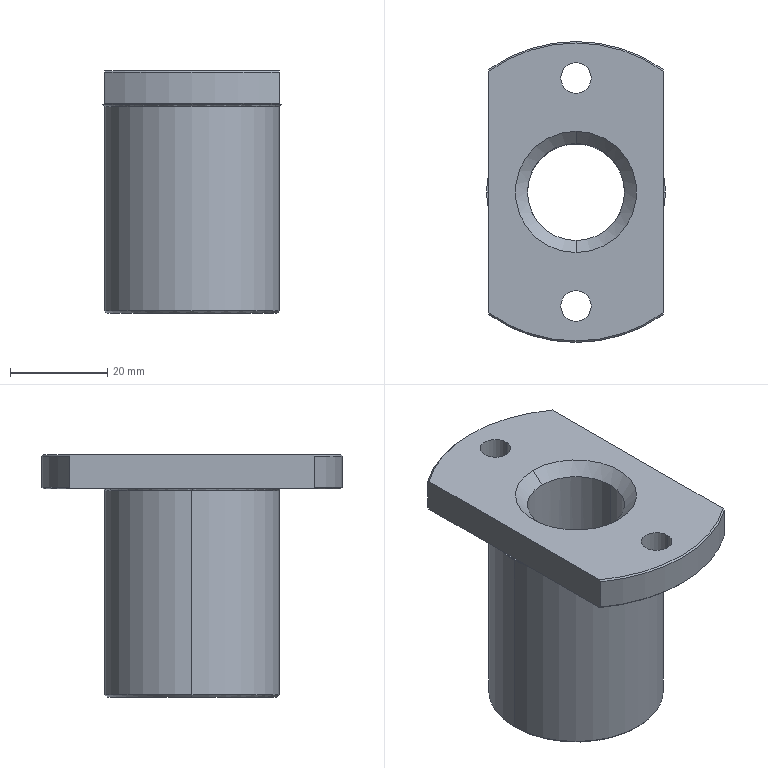Part | SolidWorks | features BaseBody 1 | 1 solid | 30 faces | box 36.8 x 62 x 50 mm | volume 41876 mm3 | cylinder 10 | cone 10 | plane 8 | spline 2 | commonest cylinder face diameters 6.3 x4 20 x2 36 x2 62 x2
STEP:
#1=CARTESIAN_POINT('',(18.4,0.,-7.));
#2=VERTEX_POINT('',#1);
#3=CARTESIAN_POINT('',(18.,3.816,-7.));
#4=VERTEX_POINT('',#3);
#5=CARTESIAN_POINT('',(18.4,0.,-7.));
#6=CARTESIAN_POINT('',(18.4,1.286,-7.));
#7=CARTESIAN_POINT('',(18.267,2.558,-7.));
#8=CARTESIAN_POINT('',(18.,3.816,-7.));
#9=B_SPLINE_CURVE_WITH_KNOTS('',3,(#5,#6,#7,#8),.UNSPECIFIED.,.F.,.F.,(4,4),(0.5,1.),.UNSPECIFIED.);
#10=EDGE_CURVE('',#2,#4,#9,.T.);
#11=ORIENTED_EDGE('',*,*,#10,.F.);
#12=CARTESIAN_POINT('',(18.,0.,-7.4));
#13=VERTEX_POINT('',#12);
#14=CARTESIAN_POINT('',(18.4,0.,-7.4));
#15=DIRECTION('',(0.,-1.,0.));
#16=DIRECTION('',(1.,0.,0.));
#17=AXIS2_PLACEMENT_3D('',#14,#15,#16);
#18=CIRCLE('',#17,0.4);
#19=EDGE_CURVE('',#2,#13,#18,.T.);
#20=ORIENTED_EDGE('',*,*,#19,.T.);
#21=CARTESIAN_POINT('',(-18.,0.,-7.4));
#22=VERTEX_POINT('',#21);
#23=CARTESIAN_POINT('',(0.,0.,-7.4));
#24=DIRECTION('',(0.,0.,-1.));
#25=DIRECTION('',(1.,0.,0.));
#26=AXIS2_PLACEMENT_3D('',#23,#24,#25);
#27=CIRCLE('',#26,18.);
#28=EDGE_CURVE('',#22,#13,#27,.T.);
#29=ORIENTED_EDGE('',*,*,#28,.F.);
#30=CARTESIAN_POINT('',(-18.4,0.,-7.));
#31=VERTEX_POINT('',#30);
#32=CARTESIAN_POINT('',(-18.4,0.,-7.4));
#33=DIRECTION('',(0.,1.,0.));
#34=DIRECTION('',(-1.,0.,0.));
#35=AXIS2_PLACEMENT_3D('',#32,#33,#34);
#36=CIRCLE('',#35,0.4);
#37=EDGE_CURVE('',#31,#22,#36,.T.);
#38=ORIENTED_EDGE('',*,*,#37,.F.);
#39=CARTESIAN_POINT('',(-18.,3.816,-7.));
#40=VERTEX_POINT('',#39);
#41=CARTESIAN_POINT('',(-18.,3.816,-7.));
#42=CARTESIAN_POINT('',(-18.267,2.558,-7.));
#43=CARTESIAN_POINT('',(-18.4,1.286,-7.));
#44=CARTESIAN_POINT('',(-18.4,0.,-7.));
#45=B_SPLINE_CURVE_WITH_KNOTS('',3,(#41,#42,#43,#44),.UNSPECIFIED.,.F.,.F.,(4,4),(0.,0.5),.UNSPECIFIED.);
#46=EDGE_CURVE('',#40,#31,#45,.T.);
#47=ORIENTED_EDGE('',*,*,#46,.F.);
#48=CARTESIAN_POINT('',(18.,3.816,-7.));
#49=CARTESIAN_POINT('',(17.897,4.302,-7.));
#50=CARTESIAN_POINT('',(17.714,5.022,-7.));
#51=CARTESIAN_POINT('',(17.45,5.846,-7.));
#52=CARTESIAN_POINT('',(17.305,6.255,-7.));
#53=CARTESIAN_POINT('',(17.229,6.458,-7.));
#54=CARTESIAN_POINT('',(17.196,6.545,-7.));
#55=CARTESIAN_POINT('',(17.174,6.603,-7.));
#56=CARTESIAN_POINT('',(17.164,6.631,-7.));
#57=CARTESIAN_POINT('',(16.964,7.145,-7.));
#58=CARTESIAN_POINT('',(16.653,7.856,-7.));
#59=CARTESIAN_POINT('',(16.238,8.66,-7.));
#60=CARTESIAN_POINT('',(16.018,9.056,-7.));
#61=CARTESIAN_POINT('',(15.921,9.224,-7.));
#62=CARTESIAN_POINT('',(15.856,9.336,-7.));
#63=CARTESIAN_POINT('',(15.824,9.39,-7.));
#64=CARTESIAN_POINT('',(15.515,9.907,-7.));
#65=CARTESIAN_POINT('',(15.074,10.575,-7.));
#66=CARTESIAN_POINT('',(14.511,11.318,-7.));
#67=CARTESIAN_POINT('',(14.26,11.629,-7.));
#68=CARTESIAN_POINT('',(14.089,11.835,-7.));
#69=CARTESIAN_POINT('',(14.005,11.935,-7.));
#70=CARTESIAN_POINT('',(13.205,12.86,-7.));
#71=CARTESIAN_POINT('',(12.428,13.612,-7.));
#72=CARTESIAN_POINT('',(11.161,14.638,-7.));
#73=CARTESIAN_POINT('',(10.508,15.122,-7.));
#74=CARTESIAN_POINT('',(9.711,15.633,-7.));
#75=CARTESIAN_POINT('',(9.362,15.841,-7.));
#76=CARTESIAN_POINT('',(9.127,15.977,-7.));
#77=CARTESIAN_POINT('',(9.008,16.045,-7.));
#78=CARTESIAN_POINT('',(8.422,16.368,-7.));
#79=CARTESIAN_POINT('',(7.705,16.724,-7.));
#80=CARTESIAN_POINT('',(6.845,17.083,-7.));
#81=CARTESIAN_POINT('',(6.408,17.249,-7.));
#82=CARTESIAN_POINT('',(6.22,17.317,-7.));
#83=CARTESIAN_POINT('',(6.094,17.362,-7.));
#84=CARTESIAN_POINT('',(6.029,17.384,-7.));
#85=CARTESIAN_POINT('',(5.477,17.574,-7.));
#86=CARTESIAN_POINT('',(4.733,17.794,-7.));
#87=CARTESIAN_POINT('',(3.851,17.996,-7.));
#88=CARTESIAN_POINT('',(3.406,18.083,-7.));
#89=CARTESIAN_POINT('',(3.183,18.123,-7.));
#90=CARTESIAN_POINT('',(3.087,18.139,-7.));
#91=CARTESIAN_POINT('',(3.023,18.15,-7.));
#92=CARTESIAN_POINT('',(2.99,18.155,-7.));
#93=CARTESIAN_POINT('',(1.979,18.32,-7.));
#94=CARTESIAN_POINT('',(0.9933,18.4,-7.));
#95=CARTESIAN_POINT('',(-0.4967,18.4,-7.));
#96=CARTESIAN_POINT('',(-1.239,18.37,-7.));
#97=CARTESIAN_POINT('',(-2.101,18.283,-7.));
#98=CARTESIAN_POINT('',(-2.531,18.226,-7.));
#99=CARTESIAN_POINT('',(-2.745,18.194,-7.));
#100=CARTESIAN_POINT('',(-2.837,18.18,-7.));
#101=CARTESIAN_POINT('',(-2.898,18.17,-7.));
#102=CARTESIAN_POINT('',(-2.927,18.166,-7.));
#103=CARTESIAN_POINT('',(-3.472,18.077,-7.));
#104=CARTESIAN_POINT('',(-4.232,17.92,-7.));
#105=CARTESIAN_POINT('',(-5.105,17.681,-7.));
#106=CARTESIAN_POINT('',(-5.537,17.548,-7.));
#107=CARTESIAN_POINT('',(-5.722,17.488,-7.));
#108=CARTESIAN_POINT('',(-5.845,17.447,-7.));
#109=CARTESIAN_POINT('',(-5.905,17.427,-7.));
#110=CARTESIAN_POINT('',(-6.474,17.232,-7.));
#111=CARTESIAN_POINT('',(-7.219,16.94,-7.));
#112=CARTESIAN_POINT('',(-8.063,16.543,-7.));
#113=CARTESIAN_POINT('',(-8.419,16.361,-7.));
#114=CARTESIAN_POINT('',(-8.656,16.237,-7.));
#115=CARTESIAN_POINT('',(-8.771,16.175,-7.));
#116=CARTESIAN_POINT('',(-9.842,15.585,-7.));
#117=CARTESIAN_POINT('',(-10.739,14.981,-7.));
#118=CARTESIAN_POINT('',(-12.006,13.954,-7.));
#119=CARTESIAN_POINT('',(-12.614,13.415,-7.));
#120=CARTESIAN_POINT('',(-13.279,12.742,-7.));
#121=CARTESIAN_POINT('',(-13.555,12.443,-7.));
#122=CARTESIAN_POINT('',(-13.737,12.242,-7.));
#123=CARTESIAN_POINT('',(-13.828,12.139,-7.));
#124=CARTESIAN_POINT('',(-14.266,11.633,-7.));
#125=CARTESIAN_POINT('',(-14.762,11.006,-7.));
#126=CARTESIAN_POINT('',(-15.292,10.239,-7.));
#127=CARTESIAN_POINT('',(-15.545,9.846,-7.));
#128=CARTESIAN_POINT('',(-15.651,9.676,-7.));
#129=CARTESIAN_POINT('',(-15.72,9.562,-7.));
#130=CARTESIAN_POINT('',(-15.756,9.503,-7.));
#131=CARTESIAN_POINT('',(-16.056,9.002,-7.));
#132=CARTESIAN_POINT('',(-16.426,8.32,-7.));
#133=CARTESIAN_POINT('',(-16.806,7.499,-7.));
#134=CARTESIAN_POINT('',(-16.983,7.082,-7.));
#135=CARTESIAN_POINT('',(-17.069,6.872,-7.));
#136=CARTESIAN_POINT('',(-17.105,6.782,-7.));
#137=CARTESIAN_POINT('',(-17.128,6.722,-7.));
#138=CARTESIAN_POINT('',(-17.141,6.69,-7.));
#139=CARTESIAN_POINT('',(-17.511,5.735,-7.));
#140=CARTESIAN_POINT('',(-17.794,4.787,-7.));
#141=CARTESIAN_POINT('',(-18.,3.816,-7.));
#142=B_SPLINE_CURVE_WITH_KNOTS('',3,(#48,#49,#50,#51,#52,#53,#54,#55,#56,#57,#58,#59,#60,#61,#62,#63,#64,#65,#66,#67,#68,#69,#70,#71,#72,#73,#74,#75,#76,#77,#78,#79,#80,#81,#82,#83,#84,#85,#86,#87,#88,#89,#90,#91,#92,#93,#94,#95,#96,#97,#98,#99,#100,#101,#102,#103,#104,#105,#106,#107,#108,#109,#110,#111,#112,#113,#114,#115,#116,#117,#118,#119,#120,#121,#122,#123,#124,#125,#126,#127,#128,#129,#130,#131,#132,#133,#134,#135,#136,#137,#138,#139,#140,#141),.UNSPECIFIED.,.F.,.F.,(4,1,1,1,1,2,2,1,1,1,2,2,1,1,2,2,2,1,1,2,2,1,1,1,2,2,1,1,1,1,2,2,2,1,1,1,1,2,2,1,1,1,2,2,1,1,2,2,2,1,1,2,2,1,1,1,2,2,1,1,1,1,2,2,4),(0.,0.03125,0.04687,0.05469,0.05859,0.06055,0.0625,0.09375,0.1094,0.1172,0.1211,0.125,0.1562,0.1719,0.1797,0.1875,0.25,0.2812,0.2969,0.3047,0.3125,0.3437,0.3594,0.3672,0.3711,0.375,0.4063,0.4219,0.4297,0.4336,0.4355,0.4375,0.5,0.5313,0.5469,0.5547,0.5586,0.5605,0.5625,0.5938,0.6094,0.6172,0.6211,0.625,0.6563,0.6719,0.6797,0.6875,0.75,0.7813,0.7969,0.8047,0.8125,0.8438,0.8594,0.8672,0.8711,0.875,0.9063,0.9219,0.9297,0.9336,0.9355,0.9375,1.),.UNSPECIFIED.);
#143=EDGE_CURVE('',#4,#40,#142,.T.);
#144=ORIENTED_EDGE('',*,*,#143,.F.);
#145=EDGE_LOOP('',(#11,#20,#29,#38,#47,#144));
#146=FACE_OUTER_BOUND('',#145,.T.);
#147=CARTESIAN_POINT('',(-18.4,0.,-7.));
#148=CARTESIAN_POINT('',(-18.4,36.8,-7.));
#149=CARTESIAN_POINT('',(18.4,36.8,-7.));
#150=CARTESIAN_POINT('',(18.4,0.,-7.));
#151=CARTESIAN_POINT('',(-18.166,0.,-7.));
#152=CARTESIAN_POINT('',(-18.166,36.331,-7.));
#153=CARTESIAN_POINT('',(18.166,36.331,-7.));
#154=CARTESIAN_POINT('',(18.166,0.,-7.));
#155=CARTESIAN_POINT('',(-18.,0.,-7.166));
#156=CARTESIAN_POINT('',(-18.,36.,-7.166));
#157=CARTESIAN_POINT('',(18.,36.,-7.166));
#158=CARTESIAN_POINT('',(18.,0.,-7.166));
#159=CARTESIAN_POINT('',(-18.,0.,-7.4));
#160=CARTESIAN_POINT('',(-18.,36.,-7.4));
#161=CARTESIAN_POINT('',(18.,36.,-7.4));
#162=CARTESIAN_POINT('',(18.,0.,-7.4));
#163=(BOUNDED_SURFACE()B_SPLINE_SURFACE(3,3,((#147,#148,#149,#150),(#151,#152,#153,#154),(#155,#156,#157,#158),(#159,#160,#161,#162)),.UNSPECIFIED.,.F.,.F.,.F.)B_SPLINE_SURFACE_WITH_KNOTS((4,4),(4,4),(0.,1.),(0.,1.),.UNSPECIFIED.)GEOMETRIC_REPRESENTATION_ITEM()RATIONAL_B_SPLINE_SURFACE(((1.,0.3333,0.3333,1.),(0.8047,0.2682,0.2682,0.8047),(0.8047,0.2682,0.2682,0.8047),(1.,0.3333,0.3333,1.)))REPRESENTATION_ITEM('')SURFACE());
#164=ADVANCED_FACE('',(#146),#163,.F.);
#165=CARTESIAN_POINT('',(18.,0.,-49.5));
#166=VERTEX_POINT('',#165);
#167=CARTESIAN_POINT('',(-18.,0.,-49.5));
#168=VERTEX_POINT('',#167);
#169=CARTESIAN_POINT('',(0.,0.,-49.5));
#170=DIRECTION('',(0.,0.,1.));
#171=DIRECTION('',(1.,0.,0.));
#172=AXIS2_PLACEMENT_3D('',#169,#170,#171);
#173=CIRCLE('',#172,18.);
#174=EDGE_CURVE('',#166,#168,#173,.T.);
#175=ORIENTED_EDGE('',*,*,#174,.T.);
#176=CARTESIAN_POINT('',(-18.,0.,-50.));
#177=DIRECTION('',(0.,0.,1.));
#178=VECTOR('',#177,1000.);
#179=LINE('',#176,#178);
#180=EDGE_CURVE('',#168,#22,#179,.T.);
#181=ORIENTED_EDGE('',*,*,#180,.T.);
#182=ORIENTED_EDGE('',*,*,#28,.T.);
#183=CARTESIAN_POINT('',(18.,0.,-50.));
#184=DIRECTION('',(0.,0.,1.));
#185=VECTOR('',#184,1000.);
#186=LINE('',#183,#185);
#187=EDGE_CURVE('',#166,#13,#186,.T.);
#188=ORIENTED_EDGE('',*,*,#187,.F.);
#189=EDGE_LOOP('',(#175,#181,#182,#188));
#190=FACE_OUTER_BOUND('',#189,.T.);
#191=CARTESIAN_POINT('',(0.,0.,-50.));
#192=DIRECTION('',(0.,0.,1.));
#193=DIRECTION('',(1.,0.,0.));
#194=AXIS2_PLACEMENT_3D('',#191,#192,#193);
#195=CYLINDRICAL_SURFACE('',#194,18.);
#196=ADVANCED_FACE('',(#190),#195,.T.);
#197=CARTESIAN_POINT('',(17.5,0.,-50.));
#198=VERTEX_POINT('',#197);
#199=CARTESIAN_POINT('',(-17.5,0.,-50.));
#200=VERTEX_POINT('',#199);
#201=CARTESIAN_POINT('',(0.,0.,-50.));
#202=DIRECTION('',(0.,0.,1.));
#203=DIRECTION('',(1.,0.,0.));
#204=AXIS2_PLACEMENT_3D('',#201,#202,#203);
#205=CIRCLE('',#204,17.5);
#206=EDGE_CURVE('',#198,#200,#205,.T.);
#207=ORIENTED_EDGE('',*,*,#206,.T.);
#208=CARTESIAN_POINT('',(-18.,0.,-49.5));
#209=DIRECTION('',(-0.7071,0.,0.7071));
#210=VECTOR('',#209,1000.);
#211=LINE('',#208,#210);
#212=EDGE_CURVE('',#200,#168,#211,.T.);
#213=ORIENTED_EDGE('',*,*,#212,.T.);
#214=ORIENTED_EDGE('',*,*,#174,.F.);
#215=CARTESIAN_POINT('',(18.,0.,-49.5));
#216=DIRECTION('',(0.7071,0.,0.7071));
#217=VECTOR('',#216,1000.);
#218=LINE('',#215,#217);
#219=EDGE_CURVE('',#198,#166,#218,.T.);
#220=ORIENTED_EDGE('',*,*,#219,.F.);
#221=EDGE_LOOP('',(#207,#213,#214,#220));
#222=FACE_OUTER_BOUND('',#221,.T.);
#223=CARTESIAN_POINT('',(0.,0.,-49.5));
#224=DIRECTION('',(0.,0.,1.));
#225=DIRECTION('',(1.,0.,0.));
#226=AXIS2_PLACEMENT_3D('',#223,#224,#225);
#227=CONICAL_SURFACE('',#226,18.,0.7854);
#228=ADVANCED_FACE('',(#222),#227,.T.);
#229=CARTESIAN_POINT('',(3.15,23.5,0.));
#230=VERTEX_POINT('',#229);
#231=CARTESIAN_POINT('',(-3.15,23.5,0.));
#232=VERTEX_POINT('',#231);
#233=CARTESIAN_POINT('',(0.,23.5,0.));
#234=DIRECTION('',(0.,0.,-1.));
#235=DIRECTION('',(-1.,0.,0.));
#236=AXIS2_PLACEMENT_3D('',#233,#234,#235);
#237=CIRCLE('',#236,3.15);
#238=EDGE_CURVE('',#230,#232,#237,.T.);
#239=ORIENTED_EDGE('',*,*,#238,.F.);
#240=CARTESIAN_POINT('',(3.15,23.5,-7.));
#241=VERTEX_POINT('',#240);
#242=CARTESIAN_POINT('',(3.15,23.5,-7.));
#243=DIRECTION('',(0.,0.,-1.));
#244=VECTOR('',#243,1000.);
#245=LINE('',#242,#244);
#246=EDGE_CURVE('',#230,#241,#245,.T.);
#247=ORIENTED_EDGE('',*,*,#246,.T.);
#248=CARTESIAN_POINT('',(-3.15,23.5,-7.));
#249=VERTEX_POINT('',#248);
#250=CARTESIAN_POINT('',(0.,23.5,-7.));
#251=DIRECTION('',(0.,0.,-1.));
#252=DIRECTION('',(-1.,0.,0.));
#253=AXIS2_PLACEMENT_3D('',#250,#251,#252);
#254=CIRCLE('',#253,3.15);
#255=EDGE_CURVE('',#241,#249,#254,.T.);
#256=ORIENTED_EDGE('',*,*,#255,.T.);
#257=CARTESIAN_POINT('',(-3.15,23.5,-7.));
#258=DIRECTION('',(0.,0.,-1.));
#259=VECTOR('',#258,1000.);
#260=LINE('',#257,#259);
#261=EDGE_CURVE('',#232,#249,#260,.T.);
#262=ORIENTED_EDGE('',*,*,#261,.F.);
#263=EDGE_LOOP('',(#239,#247,#256,#262));
#264=FACE_OUTER_BOUND('',#263,.T.);
#265=CARTESIAN_POINT('',(0.,23.5,-7.));
#266=DIRECTION('',(0.,0.,-1.));
#267=DIRECTION('',(-1.,0.,0.));
#268=AXIS2_PLACEMENT_3D('',#265,#266,#267);
#269=CYLINDRICAL_SURFACE('',#268,3.15);
#270=ADVANCED_FACE('',(#264),#269,.F.);
#271=CARTESIAN_POINT('',(3.15,-23.5,0.));
#272=VERTEX_POINT('',#271);
#273=CARTESIAN_POINT('',(-3.15,-23.5,0.));
#274=VERTEX_POINT('',#273);
#275=CARTESIAN_POINT('',(0.,-23.5,0.));
#276=DIRECTION('',(0.,0.,-1.));
#277=DIRECTION('',(-1.,0.,0.));
#278=AXIS2_PLACEMENT_3D('',#275,#276,#277);
#279=CIRCLE('',#278,3.15);
#280=EDGE_CURVE('',#272,#274,#279,.T.);
#281=ORIENTED_EDGE('',*,*,#280,.F.);
#282=CARTESIAN_POINT('',(3.15,-23.5,-7.));
#283=VERTEX_POINT('',#282);
#284=CARTESIAN_POINT('',(3.15,-23.5,-7.));
#285=DIRECTION('',(0.,0.,-1.));
#286=VECTOR('',#285,1000.);
#287=LINE('',#284,#286);
#288=EDGE_CURVE('',#272,#283,#287,.T.);
#289=ORIENTED_EDGE('',*,*,#288,.T.);
#290=CARTESIAN_POINT('',(-3.15,-23.5,-7.));
#291=VERTEX_POINT('',#290);
#292=CARTESIAN_POINT('',(0.,-23.5,-7.));
#293=DIRECTION('',(0.,0.,-1.));
#294=DIRECTION('',(-1.,0.,0.));
#295=AXIS2_PLACEMENT_3D('',#292,#293,#294);
#296=CIRCLE('',#295,3.15);
#297=EDGE_CURVE('',#283,#291,#296,.T.);
#298=ORIENTED_EDGE('',*,*,#297,.T.);
#299=CARTESIAN_POINT('',(-3.15,-23.5,-7.));
#300=DIRECTION('',(0.,0.,-1.));
#301=VECTOR('',#300,1000.);
#302=LINE('',#299,#301);
#303=EDGE_CURVE('',#274,#291,#302,.T.);
#304=ORIENTED_EDGE('',*,*,#303,.F.);
#305=EDGE_LOOP('',(#281,#289,#298,#304));
#306=FACE_OUTER_BOUND('',#305,.T.);
#307=CARTESIAN_POINT('',(0.,-23.5,-7.));
#308=DIRECTION('',(0.,0.,-1.));
#309=DIRECTION('',(-1.,0.,0.));
#310=AXIS2_PLACEMENT_3D('',#307,#308,#309);
#311=CYLINDRICAL_SURFACE('',#310,3.15);
#312=ADVANCED_FACE('',(#306),#311,.F.);
#313=CARTESIAN_POINT('',(10.,0.,-47.5));
#314=VERTEX_POINT('',#313);
#315=CARTESIAN_POINT('',(-10.,0.,-47.5));
#316=VERTEX_POINT('',#315);
#317=CARTESIAN_POINT('',(0.,0.,-47.5));
#318=DIRECTION('',(0.,0.,-1.));
#319=DIRECTION('',(-1.,0.,0.));
#320=AXIS2_PLACEMENT_3D('',#317,#318,#319);
#321=CIRCLE('',#320,10.);
#322=EDGE_CURVE('',#314,#316,#321,.T.);
#323=ORIENTED_EDGE('',*,*,#322,.F.);
#324=CARTESIAN_POINT('',(12.5,0.,-50.));
#325=VERTEX_POINT('',#324);
#326=CARTESIAN_POINT('',(12.5,0.,-50.));
#327=DIRECTION('',(0.7071,0.,-0.7071));
#328=VECTOR('',#327,1000.);
#329=LINE('',#326,#328);
#330=EDGE_CURVE('',#314,#325,#329,.T.);
#331=ORIENTED_EDGE('',*,*,#330,.T.);
#332=CARTESIAN_POINT('',(-12.5,0.,-50.));
#333=VERTEX_POINT('',#332);
#334=CARTESIAN_POINT('',(0.,0.,-50.));
#335=DIRECTION('',(0.,0.,-1.));
#336=DIRECTION('',(-1.,0.,0.));
#337=AXIS2_PLACEMENT_3D('',#334,#335,#336);
#338=CIRCLE('',#337,12.5);
#339=EDGE_CURVE('',#325,#333,#338,.T.);
#340=ORIENTED_EDGE('',*,*,#339,.T.);
#341=CARTESIAN_POINT('',(-12.5,0.,-50.));
#342=DIRECTION('',(-0.7071,0.,-0.7071));
#343=VECTOR('',#342,1000.);
#344=LINE('',#341,#343);
#345=EDGE_CURVE('',#316,#333,#344,.T.);
#346=ORIENTED_EDGE('',*,*,#345,.F.);
#347=EDGE_LOOP('',(#323,#331,#340,#346));
#348=FACE_OUTER_BOUND('',#347,.T.);
#349=CARTESIAN_POINT('',(0.,0.,-50.));
#350=DIRECTION('',(0.,0.,-1.));
#351=DIRECTION('',(-1.,0.,0.));
#352=AXIS2_PLACEMENT_3D('',#349,#350,#351);
#353=CONICAL_SURFACE('',#352,12.5,0.7854);
#354=ADVANCED_FACE('',(#348),#353,.F.);
#355=ORIENTED_EDGE('',*,*,#322,.T.);
#356=CARTESIAN_POINT('',(-10.,0.,-2.5));
#357=VERTEX_POINT('',#356);
#358=CARTESIAN_POINT('',(-10.,0.,-50.));
#359=DIRECTION('',(0.,0.,1.));
#360=VECTOR('',#359,1000.);
#361=LINE('',#358,#360);
#362=EDGE_CURVE('',#316,#357,#361,.T.);
#363=ORIENTED_EDGE('',*,*,#362,.T.);
#364=CARTESIAN_POINT('',(0.,-10.,-2.5));
#365=VERTEX_POINT('',#364);
#366=CARTESIAN_POINT('',(0.,0.,-2.5));
#367=DIRECTION('',(0.,0.,-1.));
#368=DIRECTION('',(1.,0.,0.));
#369=AXIS2_PLACEMENT_3D('',#366,#367,#368);
#370=CIRCLE('',#369,10.);
#371=EDGE_CURVE('',#365,#357,#370,.T.);
#372=ORIENTED_EDGE('',*,*,#371,.F.);
#373=CARTESIAN_POINT('',(10.,0.,-2.5));
#374=VERTEX_POINT('',#373);
#375=CARTESIAN_POINT('',(0.,0.,-2.5));
#376=DIRECTION('',(0.,0.,-1.));
#377=DIRECTION('',(1.,0.,0.));
#378=AXIS2_PLACEMENT_3D('',#375,#376,#377);
#379=CIRCLE('',#378,10.);
#380=EDGE_CURVE('',#374,#365,#379,.T.);
#381=ORIENTED_EDGE('',*,*,#380,.F.);
#382=CARTESIAN_POINT('',(10.,0.,-50.));
#383=DIRECTION('',(0.,0.,1.));
#384=VECTOR('',#383,1000.);
#385=LINE('',#382,#384);
#386=EDGE_CURVE('',#314,#374,#385,.T.);
#387=ORIENTED_EDGE('',*,*,#386,.F.);
#388=EDGE_LOOP('',(#355,#363,#372,#381,#387));
#389=FACE_OUTER_BOUND('',#388,.T.);
#390=CARTESIAN_POINT('',(0.,0.,-50.));
#391=DIRECTION('',(0.,0.,1.));
#392=DIRECTION('',(1.,0.,0.));
#393=AXIS2_PLACEMENT_3D('',#390,#391,#392);
#394=CYLINDRICAL_SURFACE('',#393,10.);
#395=ADVANCED_FACE('',(#389),#394,.F.);
#396=ORIENTED_EDGE('',*,*,#371,.T.);
#397=CARTESIAN_POINT('',(0.,10.,-2.5));
#398=VERTEX_POINT('',#397);
#399=CARTESIAN_POINT('',(0.,0.,-2.5));
#400=DIRECTION('',(0.,0.,-1.));
#401=DIRECTION('',(1.,0.,0.));
#402=AXIS2_PLACEMENT_3D('',#399,#400,#401);
#403=CIRCLE('',#402,10.);
#404=EDGE_CURVE('',#357,#398,#403,.T.);
#405=ORIENTED_EDGE('',*,*,#404,.T.);
#406=CARTESIAN_POINT('',(0.,12.5,0.));
#407=VERTEX_POINT('',#406);
#408=CARTESIAN_POINT('',(0.,12.5,0.));
#409=DIRECTION('',(0.,0.7071,0.7071));
#410=VECTOR('',#409,1000.);
#411=LINE('',#408,#410);
#412=EDGE_CURVE('',#398,#407,#411,.T.);
#413=ORIENTED_EDGE('',*,*,#412,.T.);
#414=CARTESIAN_POINT('',(0.,-12.5,0.));
#415=VERTEX_POINT('',#414);
#416=CARTESIAN_POINT('',(0.,0.,0.));
#417=DIRECTION('',(0.,0.,-1.));
#418=DIRECTION('',(0.,-1.,0.));
#419=AXIS2_PLACEMENT_3D('',#416,#417,#418);
#420=CIRCLE('',#419,12.5);
#421=EDGE_CURVE('',#415,#407,#420,.T.);
#422=ORIENTED_EDGE('',*,*,#421,.F.);
#423=CARTESIAN_POINT('',(0.,-12.5,0.));
#424=DIRECTION('',(0.,-0.7071,0.7071));
#425=VECTOR('',#424,1000.);
#426=LINE('',#423,#425);
#427=EDGE_CURVE('',#365,#415,#426,.T.);
#428=ORIENTED_EDGE('',*,*,#427,.F.);
#429=EDGE_LOOP('',(#396,#405,#413,#422,#428));
#430=FACE_OUTER_BOUND('',#429,.T.);
#431=CARTESIAN_POINT('',(0.,0.,0.));
#432=DIRECTION('',(0.,0.,1.));
#433=DIRECTION('',(0.,-1.,0.));
#434=AXIS2_PLACEMENT_3D('',#431,#432,#433);
#435=CONICAL_SURFACE('',#434,12.5,0.7854);
#436=ADVANCED_FACE('',(#430),#435,.F.);
#437=ORIENTED_EDGE('',*,*,#180,.F.);
#438=CARTESIAN_POINT('',(0.,0.,-49.5));
#439=DIRECTION('',(0.,0.,1.));
#440=DIRECTION('',(1.,0.,0.));
#441=AXIS2_PLACEMENT_3D('',#438,#439,#440);
#442=CIRCLE('',#441,18.);
#443=EDGE_CURVE('',#168,#166,#442,.T.);
#444=ORIENTED_EDGE('',*,*,#443,.T.);
#445=ORIENTED_EDGE('',*,*,#187,.T.);
#446=CARTESIAN_POINT('',(0.,0.,-7.4));
#447=DIRECTION('',(0.,0.,-1.));
#448=DIRECTION('',(1.,0.,0.));
#449=AXIS2_PLACEMENT_3D('',#446,#447,#448);
#450=CIRCLE('',#449,18.);
#451=EDGE_CURVE('',#13,#22,#450,.T.);
#452=ORIENTED_EDGE('',*,*,#451,.T.);
#453=EDGE_LOOP('',(#437,#444,#445,#452));
#454=FACE_OUTER_BOUND('',#453,.T.);
#455=CARTESIAN_POINT('',(0.,0.,-50.));
#456=DIRECTION('',(0.,0.,1.));
#457=DIRECTION('',(1.,0.,0.));
#458=AXIS2_PLACEMENT_3D('',#455,#456,#457);
#459=CYLINDRICAL_SURFACE('',#458,18.);
#460=ADVANCED_FACE('',(#454),#459,.T.);
#461=ORIENTED_EDGE('',*,*,#19,.F.);
#462=CARTESIAN_POINT('',(18.,-3.816,-7.));
#463=VERTEX_POINT('',#462);
#464=CARTESIAN_POINT('',(18.,-3.816,-7.));
#465=CARTESIAN_POINT('',(18.267,-2.558,-7.));
#466=CARTESIAN_POINT('',(18.4,-1.286,-7.));
#467=CARTESIAN_POINT('',(18.4,0.,-7.));
#468=B_SPLINE_CURVE_WITH_KNOTS('',3,(#464,#465,#466,#467),.UNSPECIFIED.,.F.,.F.,(4,4),(0.,0.5),.UNSPECIFIED.);
#469=EDGE_CURVE('',#463,#2,#468,.T.);
#470=ORIENTED_EDGE('',*,*,#469,.F.);
#471=CARTESIAN_POINT('',(-18.,-3.816,-7.));
#472=VERTEX_POINT('',#471);
#473=CARTESIAN_POINT('',(-18.,-3.816,-7.));
#474=CARTESIAN_POINT('',(-17.897,-4.302,-7.));
#475=CARTESIAN_POINT('',(-17.714,-5.022,-7.));
#476=CARTESIAN_POINT('',(-17.45,-5.846,-7.));
#477=CARTESIAN_POINT('',(-17.305,-6.255,-7.));
#478=CARTESIAN_POINT('',(-17.229,-6.458,-7.));
#479=CARTESIAN_POINT('',(-17.196,-6.545,-7.));
#480=CARTESIAN_POINT('',(-17.174,-6.603,-7.));
#481=CARTESIAN_POINT('',(-17.164,-6.631,-7.));
#482=CARTESIAN_POINT('',(-16.964,-7.145,-7.));
#483=CARTESIAN_POINT('',(-16.653,-7.856,-7.));
#484=CARTESIAN_POINT('',(-16.238,-8.66,-7.));
#485=CARTESIAN_POINT('',(-16.018,-9.056,-7.));
#486=CARTESIAN_POINT('',(-15.921,-9.224,-7.));
#487=CARTESIAN_POINT('',(-15.856,-9.336,-7.));
#488=CARTESIAN_POINT('',(-15.824,-9.39,-7.));
#489=CARTESIAN_POINT('',(-15.515,-9.907,-7.));
#490=CARTESIAN_POINT('',(-15.074,-10.575,-7.));
#491=CARTESIAN_POINT('',(-14.511,-11.318,-7.));
#492=CARTESIAN_POINT('',(-14.26,-11.629,-7.));
#493=CARTESIAN_POINT('',(-14.089,-11.835,-7.));
#494=CARTESIAN_POINT('',(-14.005,-11.935,-7.));
#495=CARTESIAN_POINT('',(-13.205,-12.86,-7.));
#496=CARTESIAN_POINT('',(-12.428,-13.612,-7.));
#497=CARTESIAN_POINT('',(-11.161,-14.638,-7.));
#498=CARTESIAN_POINT('',(-10.508,-15.122,-7.));
#499=CARTESIAN_POINT('',(-9.711,-15.633,-7.));
#500=CARTESIAN_POINT('',(-9.362,-15.841,-7.));
#501=CARTESIAN_POINT('',(-9.127,-15.977,-7.));
#502=CARTESIAN_POINT('',(-9.008,-16.045,-7.));
#503=CARTESIAN_POINT('',(-8.422,-16.368,-7.));
#504=CARTESIAN_POINT('',(-7.705,-16.724,-7.));
#505=CARTESIAN_POINT('',(-6.845,-17.083,-7.));
#506=CARTESIAN_POINT('',(-6.408,-17.249,-7.));
#507=CARTESIAN_POINT('',(-6.22,-17.317,-7.));
#508=CARTESIAN_POINT('',(-6.094,-17.362,-7.));
#509=CARTESIAN_POINT('',(-6.029,-17.384,-7.));
#510=CARTESIAN_POINT('',(-5.477,-17.574,-7.));
#511=CARTESIAN_POINT('',(-4.733,-17.794,-7.));
#512=CARTESIAN_POINT('',(-3.851,-17.996,-7.));
#513=CARTESIAN_POINT('',(-3.406,-18.083,-7.));
#514=CARTESIAN_POINT('',(-3.183,-18.123,-7.));
#515=CARTESIAN_POINT('',(-3.087,-18.139,-7.));
#516=CARTESIAN_POINT('',(-3.023,-18.15,-7.));
#517=CARTESIAN_POINT('',(-2.99,-18.155,-7.));
#518=CARTESIAN_POINT('',(-1.979,-18.32,-7.));
#519=CARTESIAN_POINT('',(-0.9933,-18.4,-7.));
#520=CARTESIAN_POINT('',(0.4967,-18.4,-7.));
#521=CARTESIAN_POINT('',(1.239,-18.37,-7.));
#522=CARTESIAN_POINT('',(2.101,-18.283,-7.));
#523=CARTESIAN_POINT('',(2.531,-18.226,-7.));
#524=CARTESIAN_POINT('',(2.745,-18.194,-7.));
#525=CARTESIAN_POINT('',(2.837,-18.18,-7.));
#526=CARTESIAN_POINT('',(2.898,-18.17,-7.));
#527=CARTESIAN_POINT('',(2.927,-18.166,-7.));
#528=CARTESIAN_POINT('',(3.472,-18.077,-7.));
#529=CARTESIAN_POINT('',(4.232,-17.92,-7.));
#530=CARTESIAN_POINT('',(5.105,-17.681,-7.));
#531=CARTESIAN_POINT('',(5.537,-17.548,-7.));
#532=CARTESIAN_POINT('',(5.722,-17.488,-7.));
#533=CARTESIAN_POINT('',(5.845,-17.447,-7.));
#534=CARTESIAN_POINT('',(5.905,-17.427,-7.));
#535=CARTESIAN_POINT('',(6.474,-17.232,-7.));
#536=CARTESIAN_POINT('',(7.219,-16.94,-7.));
#537=CARTESIAN_POINT('',(8.063,-16.543,-7.));
#538=CARTESIAN_POINT('',(8.419,-16.361,-7.));
#539=CARTESIAN_POINT('',(8.656,-16.237,-7.));
#540=CARTESIAN_POINT('',(8.771,-16.175,-7.));
#541=CARTESIAN_POINT('',(9.842,-15.585,-7.));
#542=CARTESIAN_POINT('',(10.739,-14.981,-7.));
#543=CARTESIAN_POINT('',(12.006,-13.954,-7.));
#544=CARTESIAN_POINT('',(12.614,-13.415,-7.));
#545=CARTESIAN_POINT('',(13.279,-12.742,-7.));
#546=CARTESIAN_POINT('',(13.555,-12.443,-7.));
#547=CARTESIAN_POINT('',(13.737,-12.242,-7.));
#548=CARTESIAN_POINT('',(13.828,-12.139,-7.));
#549=CARTESIAN_POINT('',(14.266,-11.633,-7.));
#550=CARTESIAN_POINT('',(14.762,-11.006,-7.));
#551=CARTESIAN_POINT('',(15.292,-10.239,-7.));
#552=CARTESIAN_POINT('',(15.545,-9.846,-7.));
#553=CARTESIAN_POINT('',(15.651,-9.676,-7.));
#554=CARTESIAN_POINT('',(15.72,-9.562,-7.));
#555=CARTESIAN_POINT('',(15.756,-9.503,-7.));
#556=CARTESIAN_POINT('',(16.056,-9.002,-7.));
#557=CARTESIAN_POINT('',(16.426,-8.32,-7.));
#558=CARTESIAN_POINT('',(16.806,-7.499,-7.));
#559=CARTESIAN_POINT('',(16.983,-7.082,-7.));
#560=CARTESIAN_POINT('',(17.069,-6.872,-7.));
#561=CARTESIAN_POINT('',(17.105,-6.782,-7.));
#562=CARTESIAN_POINT('',(17.128,-6.722,-7.));
#563=CARTESIAN_POINT('',(17.141,-6.69,-7.));
#564=CARTESIAN_POINT('',(17.511,-5.735,-7.));
#565=CARTESIAN_POINT('',(17.794,-4.787,-7.));
#566=CARTESIAN_POINT('',(18.,-3.816,-7.));
#567=B_SPLINE_CURVE_WITH_KNOTS('',3,(#473,#474,#475,#476,#477,#478,#479,#480,#481,#482,#483,#484,#485,#486,#487,#488,#489,#490,#491,#492,#493,#494,#495,#496,#497,#498,#499,#500,#501,#502,#503,#504,#505,#506,#507,#508,#509,#510,#511,#512,#513,#514,#515,#516,#517,#518,#519,#520,#521,#522,#523,#524,#525,#526,#527,#528,#529,#530,#531,#532,#533,#534,#535,#536,#537,#538,#539,#540,#541,#542,#543,#544,#545,#546,#547,#548,#549,#550,#551,#552,#553,#554,#555,#556,#557,#558,#559,#560,#561,#562,#563,#564,#565,#566),.UNSPECIFIED.,.F.,.F.,(4,1,1,1,1,2,2,1,1,1,2,2,1,1,2,2,2,1,1,2,2,1,1,1,2,2,1,1,1,1,2,2,2,1,1,1,1,2,2,1,1,1,2,2,1,1,2,2,2,1,1,2,2,1,1,1,2,2,1,1,1,1,2,2,4),(0.,0.03125,0.04687,0.05469,0.05859,0.06055,0.0625,0.09375,0.1094,0.1172,0.1211,0.125,0.1562,0.1719,0.1797,0.1875,0.25,0.2812,0.2969,0.3047,0.3125,0.3437,0.3594,0.3672,0.3711,0.375,0.4062,0.4219,0.4297,0.4336,0.4355,0.4375,0.5,0.5312,0.5469,0.5547,0.5586,0.5605,0.5625,0.5937,0.6094,0.6172,0.6211,0.625,0.6562,0.6719,0.6797,0.6875,0.75,0.7812,0.7969,0.8047,0.8125,0.8437,0.8594,0.8672,0.8711,0.875,0.9062,0.9219,0.9297,0.9336,0.9355,0.9375,1.),.UNSPECIFIED.);
#568=EDGE_CURVE('',#472,#463,#567,.T.);
#569=ORIENTED_EDGE('',*,*,#568,.F.);
#570=CARTESIAN_POINT('',(-18.4,0.,-7.));
#571=CARTESIAN_POINT('',(-18.4,-1.286,-7.));
#572=CARTESIAN_POINT('',(-18.267,-2.558,-7.));
#573=CARTESIAN_POINT('',(-18.,-3.816,-7.));
#574=B_SPLINE_CURVE_WITH_KNOTS('',3,(#570,#571,#572,#573),.UNSPECIFIED.,.F.,.F.,(4,4),(0.5,1.),.UNSPECIFIED.);
#575=EDGE_CURVE('',#31,#472,#574,.T.);
#576=ORIENTED_EDGE('',*,*,#575,.F.);
#577=ORIENTED_EDGE('',*,*,#37,.T.);
#578=ORIENTED_EDGE('',*,*,#451,.F.);
#579=EDGE_LOOP('',(#461,#470,#569,#576,#577,#578));
#580=FACE_OUTER_BOUND('',#579,.T.);
#581=CARTESIAN_POINT('',(18.4,0.,-7.));
#582=CARTESIAN_POINT('',(18.4,-36.8,-7.));
#583=CARTESIAN_POINT('',(-18.4,-36.8,-7.));
#584=CARTESIAN_POINT('',(-18.4,0.,-7.));
#585=CARTESIAN_POINT('',(18.166,0.,-7.));
#586=CARTESIAN_POINT('',(18.166,-36.331,-7.));
#587=CARTESIAN_POINT('',(-18.166,-36.331,-7.));
#588=CARTESIAN_POINT('',(-18.166,0.,-7.));
#589=CARTESIAN_POINT('',(18.,0.,-7.166));
#590=CARTESIAN_POINT('',(18.,-36.,-7.166));
#591=CARTESIAN_POINT('',(-18.,-36.,-7.166));
#592=CARTESIAN_POINT('',(-18.,0.,-7.166));
#593=CARTESIAN_POINT('',(18.,0.,-7.4));
#594=CARTESIAN_POINT('',(18.,-36.,-7.4));
#595=CARTESIAN_POINT('',(-18.,-36.,-7.4));
#596=CARTESIAN_POINT('',(-18.,0.,-7.4));
#597=(BOUNDED_SURFACE()B_SPLINE_SURFACE(3,3,((#581,#582,#583,#584),(#585,#586,#587,#588),(#589,#590,#591,#592),(#593,#594,#595,#596)),.UNSPECIFIED.,.F.,.F.,.T.)B_SPLINE_SURFACE_WITH_KNOTS((4,4),(4,4),(0.,1.),(0.,1.),.UNSPECIFIED.)GEOMETRIC_REPRESENTATION_ITEM()RATIONAL_B_SPLINE_SURFACE(((1.,0.3333,0.3333,1.),(0.8047,0.2682,0.2682,0.8047),(0.8047,0.2682,0.2682,0.8047),(1.,0.3333,0.3333,1.)))REPRESENTATION_ITEM('')SURFACE());
#598=ADVANCED_FACE('',(#580),#597,.F.);
#599=ORIENTED_EDGE('',*,*,#212,.F.);
#600=CARTESIAN_POINT('',(0.,0.,-50.));
#601=DIRECTION('',(0.,0.,1.));
#602=DIRECTION('',(1.,0.,0.));
#603=AXIS2_PLACEMENT_3D('',#600,#601,#602);
#604=CIRCLE('',#603,17.5);
#605=EDGE_CURVE('',#200,#198,#604,.T.);
#606=ORIENTED_EDGE('',*,*,#605,.T.);
#607=ORIENTED_EDGE('',*,*,#219,.T.);
#608=ORIENTED_EDGE('',*,*,#443,.F.);
#609=EDGE_LOOP('',(#599,#606,#607,#608));
#610=FACE_OUTER_BOUND('',#609,.T.);
#611=CARTESIAN_POINT('',(0.,0.,-49.5));
#612=DIRECTION('',(0.,0.,1.));
#613=DIRECTION('',(1.,0.,0.));
#614=AXIS2_PLACEMENT_3D('',#611,#612,#613);
#615=CONICAL_SURFACE('',#614,18.,0.7854);
#616=ADVANCED_FACE('',(#610),#615,.T.);
#617=CARTESIAN_POINT('',(-18.,0.,-7.));
#618=DIRECTION('',(0.,-1.,0.));
#619=VECTOR('',#618,1000.);
#620=LINE('',#617,#619);
#621=EDGE_CURVE('',#40,#472,#620,.T.);
#622=ORIENTED_EDGE('',*,*,#621,.F.);
#623=ORIENTED_EDGE('',*,*,#46,.T.);
#624=ORIENTED_EDGE('',*,*,#575,.T.);
#625=EDGE_LOOP('',(#622,#623,#624));
#626=FACE_OUTER_BOUND('',#625,.T.);
#627=CARTESIAN_POINT('',(0.,0.,-7.));
#628=DIRECTION('',(0.,0.,-1.));
#629=DIRECTION('',(-1.,0.,0.));
#630=AXIS2_PLACEMENT_3D('',#627,#628,#629);
#631=PLANE('',#630);
#632=ADVANCED_FACE('',(#626),#631,.F.);
#633=CARTESIAN_POINT('',(18.,24.869,-7.));
#634=VERTEX_POINT('',#633);
#635=CARTESIAN_POINT('',(18.,0.,-7.));
#636=DIRECTION('',(0.,1.,0.));
#637=VECTOR('',#636,1000.);
#638=LINE('',#635,#637);
#639=EDGE_CURVE('',#4,#634,#638,.T.);
#640=ORIENTED_EDGE('',*,*,#639,.F.);
#641=ORIENTED_EDGE('',*,*,#143,.T.);
#642=CARTESIAN_POINT('',(-18.,24.869,-7.));
#643=VERTEX_POINT('',#642);
#644=CARTESIAN_POINT('',(-18.,0.,-7.));
#645=DIRECTION('',(0.,-1.,0.));
#646=VECTOR('',#645,1000.);
#647=LINE('',#644,#646);
#648=EDGE_CURVE('',#643,#40,#647,.T.);
#649=ORIENTED_EDGE('',*,*,#648,.F.);
#650=CARTESIAN_POINT('',(0.,0.,-7.));
#651=DIRECTION('',(0.,0.,1.));
#652=DIRECTION('',(0.,-1.,0.));
#653=AXIS2_PLACEMENT_3D('',#650,#651,#652);
#654=CIRCLE('',#653,30.7);
#655=EDGE_CURVE('',#634,#643,#654,.T.);
#656=ORIENTED_EDGE('',*,*,#655,.F.);
#657=EDGE_LOOP('',(#640,#641,#649,#656));
#658=FACE_OUTER_BOUND('',#657,.T.);
#659=CARTESIAN_POINT('',(0.,23.5,-7.));
#660=DIRECTION('',(0.,0.,-1.));
#661=DIRECTION('',(-1.,0.,0.));
#662=AXIS2_PLACEMENT_3D('',#659,#660,#661);
#663=CIRCLE('',#662,3.15);
#664=EDGE_CURVE('',#249,#241,#663,.T.);
#665=ORIENTED_EDGE('',*,*,#664,.F.);
#666=ORIENTED_EDGE('',*,*,#255,.F.);
#667=EDGE_LOOP('',(#665,#666));
#668=FACE_BOUND('',#667,.T.);
#669=CARTESIAN_POINT('',(0.,0.,-7.));
#670=DIRECTION('',(0.,0.,1.));
#671=DIRECTION('',(1.,0.,0.));
#672=AXIS2_PLACEMENT_3D('',#669,#670,#671);
#673=PLANE('',#672);
#674=ADVANCED_FACE('',(#658,#668),#673,.F.);
#675=CARTESIAN_POINT('',(18.,0.,-7.));
#676=DIRECTION('',(0.,1.,0.));
#677=VECTOR('',#676,1000.);
#678=LINE('',#675,#677);
#679=EDGE_CURVE('',#463,#4,#678,.T.);
#680=ORIENTED_EDGE('',*,*,#679,.F.);
#681=ORIENTED_EDGE('',*,*,#469,.T.);
#682=ORIENTED_EDGE('',*,*,#10,.T.);
#683=EDGE_LOOP('',(#680,#681,#682));
#684=FACE_OUTER_BOUND('',#683,.T.);
#685=CARTESIAN_POINT('',(0.,0.,-7.));
#686=DIRECTION('',(0.,0.,-1.));
#687=DIRECTION('',(-1.,0.,0.));
#688=AXIS2_PLACEMENT_3D('',#685,#686,#687);
#689=PLANE('',#688);
#690=ADVANCED_FACE('',(#684),#689,.F.);
#691=CARTESIAN_POINT('',(-18.,-24.869,-7.));
#692=VERTEX_POINT('',#691);
#693=CARTESIAN_POINT('',(18.,-24.869,-7.));
#694=VERTEX_POINT('',#693);
#695=CARTESIAN_POINT('',(0.,0.,-7.));
#696=DIRECTION('',(0.,0.,1.));
#697=DIRECTION('',(1.,0.,0.));
#698=AXIS2_PLACEMENT_3D('',#695,#696,#697);
#699=CIRCLE('',#698,30.7);
#700=EDGE_CURVE('',#692,#694,#699,.T.);
#701=ORIENTED_EDGE('',*,*,#700,.F.);
#702=CARTESIAN_POINT('',(-18.,0.,-7.));
#703=DIRECTION('',(0.,-1.,0.));
#704=VECTOR('',#703,1000.);
#705=LINE('',#702,#704);
#706=EDGE_CURVE('',#472,#692,#705,.T.);
#707=ORIENTED_EDGE('',*,*,#706,.F.);
#708=ORIENTED_EDGE('',*,*,#568,.T.);
#709=CARTESIAN_POINT('',(18.,0.,-7.));
#710=DIRECTION('',(0.,1.,0.));
#711=VECTOR('',#710,1000.);
#712=LINE('',#709,#711);
#713=EDGE_CURVE('',#694,#463,#712,.T.);
#714=ORIENTED_EDGE('',*,*,#713,.F.);
#715=EDGE_LOOP('',(#701,#707,#708,#714));
#716=FACE_OUTER_BOUND('',#715,.T.);
#717=CARTESIAN_POINT('',(0.,-23.5,-7.));
#718=DIRECTION('',(0.,0.,-1.));
#719=DIRECTION('',(-1.,0.,0.));
#720=AXIS2_PLACEMENT_3D('',#717,#718,#719);
#721=CIRCLE('',#720,3.15);
#722=EDGE_CURVE('',#291,#283,#721,.T.);
#723=ORIENTED_EDGE('',*,*,#722,.F.);
#724=ORIENTED_EDGE('',*,*,#297,.F.);
#725=EDGE_LOOP('',(#723,#724));
#726=FACE_BOUND('',#725,.T.);
#727=CARTESIAN_POINT('',(0.,0.,-7.));
#728=DIRECTION('',(0.,0.,1.));
#729=DIRECTION('',(1.,0.,0.));
#730=AXIS2_PLACEMENT_3D('',#727,#728,#729);
#731=PLANE('',#730);
#732=ADVANCED_FACE('',(#716,#726),#731,.F.);
#733=ORIENTED_EDGE('',*,*,#206,.F.);
#734=ORIENTED_EDGE('',*,*,#605,.F.);
#735=EDGE_LOOP('',(#733,#734));
#736=FACE_OUTER_BOUND('',#735,.T.);
#737=CARTESIAN_POINT('',(0.,0.,-50.));
#738=DIRECTION('',(0.,0.,-1.));
#739=DIRECTION('',(-1.,0.,0.));
#740=AXIS2_PLACEMENT_3D('',#737,#738,#739);
#741=CIRCLE('',#740,12.5);
#742=EDGE_CURVE('',#333,#325,#741,.T.);
#743=ORIENTED_EDGE('',*,*,#742,.F.);
#744=ORIENTED_EDGE('',*,*,#339,.F.);
#745=EDGE_LOOP('',(#743,#744));
#746=FACE_BOUND('',#745,.T.);
#747=CARTESIAN_POINT('',(0.,17.5,-50.));
#748=DIRECTION('',(0.,0.,1.));
#749=DIRECTION('',(1.,0.,0.));
#750=AXIS2_PLACEMENT_3D('',#747,#748,#749);
#751=PLANE('',#750);
#752=ADVANCED_FACE('',(#736,#746),#751,.F.);
#753=ORIENTED_EDGE('',*,*,#621,.T.);
#754=ORIENTED_EDGE('',*,*,#706,.T.);
#755=CARTESIAN_POINT('',(-18.,-25.239,-6.7));
#756=VERTEX_POINT('',#755);
#757=CARTESIAN_POINT('',(-18.,-24.869,-7.));
#758=CARTESIAN_POINT('',(-18.,-24.993,-6.9));
#759=CARTESIAN_POINT('',(-18.,-25.116,-6.8));
#760=CARTESIAN_POINT('',(-18.,-25.239,-6.7));
#761=B_SPLINE_CURVE_WITH_KNOTS('',3,(#757,#758,#759,#760),.UNSPECIFIED.,.F.,.F.,(4,4),(0.,0.0004759),.UNSPECIFIED.);
#762=EDGE_CURVE('',#692,#756,#761,.T.);
#763=ORIENTED_EDGE('',*,*,#762,.T.);
#764=CARTESIAN_POINT('',(-18.,-25.239,-0.3));
#765=VERTEX_POINT('',#764);
#766=CARTESIAN_POINT('',(-18.,-25.239,-7.));
#767=DIRECTION('',(0.,0.,1.));
#768=VECTOR('',#767,1000.);
#769=LINE('',#766,#768);
#770=EDGE_CURVE('',#756,#765,#769,.T.);
#771=ORIENTED_EDGE('',*,*,#770,.T.);
#772=CARTESIAN_POINT('',(-18.,-24.869,0.));
#773=VERTEX_POINT('',#772);
#774=CARTESIAN_POINT('',(-18.,-24.869,0.));
#775=CARTESIAN_POINT('',(-18.,-24.993,-0.09985));
#776=CARTESIAN_POINT('',(-18.,-25.116,-0.1998));
#777=CARTESIAN_POINT('',(-18.,-25.239,-0.3));
#778=B_SPLINE_CURVE_WITH_KNOTS('',3,(#774,#775,#776,#777),.UNSPECIFIED.,.F.,.F.,(4,4),(0.,0.0004759),.UNSPECIFIED.);
#779=EDGE_CURVE('',#773,#765,#778,.T.);
#780=ORIENTED_EDGE('',*,*,#779,.F.);
#781=CARTESIAN_POINT('',(-18.,24.869,0.));
#782=VERTEX_POINT('',#781);
#783=CARTESIAN_POINT('',(-18.,25.239,0.));
#784=DIRECTION('',(0.,1.,0.));
#785=VECTOR('',#784,1000.);
#786=LINE('',#783,#785);
#787=EDGE_CURVE('',#773,#782,#786,.T.);
#788=ORIENTED_EDGE('',*,*,#787,.T.);
#789=CARTESIAN_POINT('',(-18.,25.239,-0.3));
#790=VERTEX_POINT('',#789);
#791=CARTESIAN_POINT('',(-18.,25.239,-0.3));
#792=CARTESIAN_POINT('',(-18.,25.116,-0.1998));
#793=CARTESIAN_POINT('',(-18.,24.993,-0.09985));
#794=CARTESIAN_POINT('',(-18.,24.869,0.));
#795=B_SPLINE_CURVE_WITH_KNOTS('',3,(#791,#792,#793,#794),.UNSPECIFIED.,.F.,.F.,(4,4),(0.,0.0004759),.UNSPECIFIED.);
#796=EDGE_CURVE('',#790,#782,#795,.T.);
#797=ORIENTED_EDGE('',*,*,#796,.F.);
#798=CARTESIAN_POINT('',(-18.,25.239,-6.7));
#799=VERTEX_POINT('',#798);
#800=CARTESIAN_POINT('',(-18.,25.239,-7.));
#801=DIRECTION('',(0.,0.,-1.));
#802=VECTOR('',#801,1000.);
#803=LINE('',#800,#802);
#804=EDGE_CURVE('',#790,#799,#803,.T.);
#805=ORIENTED_EDGE('',*,*,#804,.T.);
#806=CARTESIAN_POINT('',(-18.,25.239,-6.7));
#807=CARTESIAN_POINT('',(-18.,25.116,-6.8));
#808=CARTESIAN_POINT('',(-18.,24.993,-6.9));
#809=CARTESIAN_POINT('',(-18.,24.869,-7.));
#810=B_SPLINE_CURVE_WITH_KNOTS('',3,(#806,#807,#808,#809),.UNSPECIFIED.,.F.,.F.,(4,4),(0.,0.0004759),.UNSPECIFIED.);
#811=EDGE_CURVE('',#799,#643,#810,.T.);
#812=ORIENTED_EDGE('',*,*,#811,.T.);
#813=ORIENTED_EDGE('',*,*,#648,.T.);
#814=EDGE_LOOP('',(#753,#754,#763,#771,#780,#788,#797,#805,#812,#813));
#815=FACE_OUTER_BOUND('',#814,.T.);
#816=CARTESIAN_POINT('',(-18.,25.239,-7.));
#817=DIRECTION('',(-1.,0.,0.));
#818=DIRECTION('',(0.,0.,1.));
#819=AXIS2_PLACEMENT_3D('',#816,#817,#818);
#820=PLANE('',#819);
#821=ADVANCED_FACE('',(#815),#820,.T.);
#822=CARTESIAN_POINT('',(18.,25.239,-6.7));
#823=VERTEX_POINT('',#822);
#824=CARTESIAN_POINT('',(18.,25.239,-6.7));
#825=CARTESIAN_POINT('',(18.,25.116,-6.8));
#826=CARTESIAN_POINT('',(18.,24.993,-6.9));
#827=CARTESIAN_POINT('',(18.,24.869,-7.));
#828=B_SPLINE_CURVE_WITH_KNOTS('',3,(#824,#825,#826,#827),.UNSPECIFIED.,.F.,.F.,(4,4),(0.,0.0004759),.UNSPECIFIED.);
#829=EDGE_CURVE('',#823,#634,#828,.T.);
#830=ORIENTED_EDGE('',*,*,#829,.T.);
#831=ORIENTED_EDGE('',*,*,#655,.T.);
#832=ORIENTED_EDGE('',*,*,#811,.F.);
#833=CARTESIAN_POINT('',(0.,0.,-6.7));
#834=DIRECTION('',(0.,0.,-1.));
#835=DIRECTION('',(1.,0.,0.));
#836=AXIS2_PLACEMENT_3D('',#833,#834,#835);
#837=CIRCLE('',#836,31.);
#838=EDGE_CURVE('',#799,#823,#837,.T.);
#839=ORIENTED_EDGE('',*,*,#838,.T.);
#840=EDGE_LOOP('',(#830,#831,#832,#839));
#841=FACE_OUTER_BOUND('',#840,.T.);
#842=CARTESIAN_POINT('',(0.,0.,-6.7));
#843=DIRECTION('',(0.,0.,1.));
#844=DIRECTION('',(0.,-1.,0.));
#845=AXIS2_PLACEMENT_3D('',#842,#843,#844);
#846=CONICAL_SURFACE('',#845,31.,0.7854);
#847=ADVANCED_FACE('',(#841),#846,.T.);
#848=ORIENTED_EDGE('',*,*,#679,.T.);
#849=ORIENTED_EDGE('',*,*,#639,.T.);
#850=ORIENTED_EDGE('',*,*,#829,.F.);
#851=CARTESIAN_POINT('',(18.,25.239,-0.3));
#852=VERTEX_POINT('',#851);
#853=CARTESIAN_POINT('',(18.,25.239,-7.));
#854=DIRECTION('',(0.,0.,1.));
#855=VECTOR('',#854,1000.);
#856=LINE('',#853,#855);
#857=EDGE_CURVE('',#823,#852,#856,.T.);
#858=ORIENTED_EDGE('',*,*,#857,.T.);
#859=CARTESIAN_POINT('',(18.,24.869,0.));
#860=VERTEX_POINT('',#859);
#861=CARTESIAN_POINT('',(18.,24.869,0.));
#862=CARTESIAN_POINT('',(18.,24.993,-0.09985));
#863=CARTESIAN_POINT('',(18.,25.116,-0.1998));
#864=CARTESIAN_POINT('',(18.,25.239,-0.3));
#865=B_SPLINE_CURVE_WITH_KNOTS('',3,(#861,#862,#863,#864),.UNSPECIFIED.,.F.,.F.,(4,4),(0.,0.0004759),.UNSPECIFIED.);
#866=EDGE_CURVE('',#860,#852,#865,.T.);
#867=ORIENTED_EDGE('',*,*,#866,.F.);
#868=CARTESIAN_POINT('',(18.,-24.869,0.));
#869=VERTEX_POINT('',#868);
#870=CARTESIAN_POINT('',(18.,-25.239,0.));
#871=DIRECTION('',(0.,-1.,0.));
#872=VECTOR('',#871,1000.);
#873=LINE('',#870,#872);
#874=EDGE_CURVE('',#860,#869,#873,.T.);
#875=ORIENTED_EDGE('',*,*,#874,.T.);
#876=CARTESIAN_POINT('',(18.,-25.239,-0.3));
#877=VERTEX_POINT('',#876);
#878=CARTESIAN_POINT('',(18.,-25.239,-0.3));
#879=CARTESIAN_POINT('',(18.,-25.116,-0.1998));
#880=CARTESIAN_POINT('',(18.,-24.993,-0.09985));
#881=CARTESIAN_POINT('',(18.,-24.869,0.));
#882=B_SPLINE_CURVE_WITH_KNOTS('',3,(#878,#879,#880,#881),.UNSPECIFIED.,.F.,.F.,(4,4),(0.,0.0004759),.UNSPECIFIED.);
#883=EDGE_CURVE('',#877,#869,#882,.T.);
#884=ORIENTED_EDGE('',*,*,#883,.F.);
#885=CARTESIAN_POINT('',(18.,-25.239,-6.7));
#886=VERTEX_POINT('',#885);
#887=CARTESIAN_POINT('',(18.,-25.239,-7.));
#888=DIRECTION('',(0.,0.,-1.));
#889=VECTOR('',#888,1000.);
#890=LINE('',#887,#889);
#891=EDGE_CURVE('',#877,#886,#890,.T.);
#892=ORIENTED_EDGE('',*,*,#891,.T.);
#893=CARTESIAN_POINT('',(18.,-25.239,-6.7));
#894=CARTESIAN_POINT('',(18.,-25.116,-6.8));
#895=CARTESIAN_POINT('',(18.,-24.993,-6.9));
#896=CARTESIAN_POINT('',(18.,-24.869,-7.));
#897=B_SPLINE_CURVE_WITH_KNOTS('',3,(#893,#894,#895,#896),.UNSPECIFIED.,.F.,.F.,(4,4),(0.,0.0004759),.UNSPECIFIED.);
#898=EDGE_CURVE('',#886,#694,#897,.T.);
#899=ORIENTED_EDGE('',*,*,#898,.T.);
#900=ORIENTED_EDGE('',*,*,#713,.T.);
#901=EDGE_LOOP('',(#848,#849,#850,#858,#867,#875,#884,#892,#899,#900));
#902=FACE_OUTER_BOUND('',#901,.T.);
#903=CARTESIAN_POINT('',(18.,-25.239,-7.));
#904=DIRECTION('',(1.,0.,0.));
#905=DIRECTION('',(0.,0.,-1.));
#906=AXIS2_PLACEMENT_3D('',#903,#904,#905);
#907=PLANE('',#906);
#908=ADVANCED_FACE('',(#902),#907,.T.);
#909=ORIENTED_EDGE('',*,*,#246,.F.);
#910=CARTESIAN_POINT('',(0.,23.5,0.));
#911=DIRECTION('',(0.,0.,-1.));
#912=DIRECTION('',(-1.,0.,0.));
#913=AXIS2_PLACEMENT_3D('',#910,#911,#912);
#914=CIRCLE('',#913,3.15);
#915=EDGE_CURVE('',#232,#230,#914,.T.);
#916=ORIENTED_EDGE('',*,*,#915,.F.);
#917=ORIENTED_EDGE('',*,*,#261,.T.);
#918=ORIENTED_EDGE('',*,*,#664,.T.);
#919=EDGE_LOOP('',(#909,#916,#917,#918));
#920=FACE_OUTER_BOUND('',#919,.T.);
#921=CARTESIAN_POINT('',(0.,23.5,-7.));
#922=DIRECTION('',(0.,0.,-1.));
#923=DIRECTION('',(-1.,0.,0.));
#924=AXIS2_PLACEMENT_3D('',#921,#922,#923);
#925=CYLINDRICAL_SURFACE('',#924,3.15);
#926=ADVANCED_FACE('',(#920),#925,.F.);
#927=ORIENTED_EDGE('',*,*,#898,.F.);
#928=CARTESIAN_POINT('',(0.,0.,-6.7));
#929=DIRECTION('',(0.,0.,-1.));
#930=DIRECTION('',(1.,0.,0.));
#931=AXIS2_PLACEMENT_3D('',#928,#929,#930);
#932=CIRCLE('',#931,31.);
#933=EDGE_CURVE('',#886,#756,#932,.T.);
#934=ORIENTED_EDGE('',*,*,#933,.T.);
#935=ORIENTED_EDGE('',*,*,#762,.F.);
#936=ORIENTED_EDGE('',*,*,#700,.T.);
#937=EDGE_LOOP('',(#927,#934,#935,#936));
#938=FACE_OUTER_BOUND('',#937,.T.);
#939=CARTESIAN_POINT('',(0.,0.,-6.7));
#940=DIRECTION('',(0.,0.,1.));
#941=DIRECTION('',(1.,0.,0.));
#942=AXIS2_PLACEMENT_3D('',#939,#940,#941);
#943=CONICAL_SURFACE('',#942,31.,0.7854);
#944=ADVANCED_FACE('',(#938),#943,.T.);
#945=ORIENTED_EDGE('',*,*,#288,.F.);
#946=CARTESIAN_POINT('',(0.,-23.5,0.));
#947=DIRECTION('',(0.,0.,-1.));
#948=DIRECTION('',(-1.,0.,0.));
#949=AXIS2_PLACEMENT_3D('',#946,#947,#948);
#950=CIRCLE('',#949,3.15);
#951=EDGE_CURVE('',#274,#272,#950,.T.);
#952=ORIENTED_EDGE('',*,*,#951,.F.);
#953=ORIENTED_EDGE('',*,*,#303,.T.);
#954=ORIENTED_EDGE('',*,*,#722,.T.);
#955=EDGE_LOOP('',(#945,#952,#953,#954));
#956=FACE_OUTER_BOUND('',#955,.T.);
#957=CARTESIAN_POINT('',(0.,-23.5,-7.));
#958=DIRECTION('',(0.,0.,-1.));
#959=DIRECTION('',(-1.,0.,0.));
#960=AXIS2_PLACEMENT_3D('',#957,#958,#959);
#961=CYLINDRICAL_SURFACE('',#960,3.15);
#962=ADVANCED_FACE('',(#956),#961,.F.);
#963=ORIENTED_EDGE('',*,*,#330,.F.);
#964=CARTESIAN_POINT('',(0.,0.,-47.5));
#965=DIRECTION('',(0.,0.,-1.));
#966=DIRECTION('',(-1.,0.,0.));
#967=AXIS2_PLACEMENT_3D('',#964,#965,#966);
#968=CIRCLE('',#967,10.);
#969=EDGE_CURVE('',#316,#314,#968,.T.);
#970=ORIENTED_EDGE('',*,*,#969,.F.);
#971=ORIENTED_EDGE('',*,*,#345,.T.);
#972=ORIENTED_EDGE('',*,*,#742,.T.);
#973=EDGE_LOOP('',(#963,#970,#971,#972));
#974=FACE_OUTER_BOUND('',#973,.T.);
#975=CARTESIAN_POINT('',(0.,0.,-50.));
#976=DIRECTION('',(0.,0.,-1.));
#977=DIRECTION('',(-1.,0.,0.));
#978=AXIS2_PLACEMENT_3D('',#975,#976,#977);
#979=CONICAL_SURFACE('',#978,12.5,0.7854);
#980=ADVANCED_FACE('',(#974),#979,.F.);
#981=ORIENTED_EDGE('',*,*,#804,.F.);
#982=CARTESIAN_POINT('',(0.,0.,-0.3));
#983=DIRECTION('',(0.,0.,-1.));
#984=DIRECTION('',(-1.,0.,0.));
#985=AXIS2_PLACEMENT_3D('',#982,#983,#984);
#986=CIRCLE('',#985,31.);
#987=EDGE_CURVE('',#790,#852,#986,.T.);
#988=ORIENTED_EDGE('',*,*,#987,.T.);
#989=ORIENTED_EDGE('',*,*,#857,.F.);
#990=ORIENTED_EDGE('',*,*,#838,.F.);
#991=EDGE_LOOP('',(#981,#988,#989,#990));
#992=FACE_OUTER_BOUND('',#991,.T.);
#993=CARTESIAN_POINT('',(0.,0.,-7.));
#994=DIRECTION('',(0.,0.,-1.));
#995=DIRECTION('',(-1.,0.,0.));
#996=AXIS2_PLACEMENT_3D('',#993,#994,#995);
#997=CYLINDRICAL_SURFACE('',#996,31.);
#998=ADVANCED_FACE('',(#992),#997,.T.);
#999=ORIENTED_EDGE('',*,*,#421,.T.);
#1000=CARTESIAN_POINT('',(0.,0.,0.));
#1001=DIRECTION('',(0.,0.,-1.));
#1002=DIRECTION('',(0.,-1.,0.));
#1003=AXIS2_PLACEMENT_3D('',#1000,#1001,#1002);
#1004=CIRCLE('',#1003,12.5);
#1005=EDGE_CURVE('',#407,#415,#1004,.T.);
#1006=ORIENTED_EDGE('',*,*,#1005,.T.);
#1007=EDGE_LOOP('',(#999,#1006));
#1008=FACE_BOUND('',#1007,.T.);
#1009=ORIENTED_EDGE('',*,*,#915,.T.);
#1010=ORIENTED_EDGE('',*,*,#238,.T.);
#1011=EDGE_LOOP('',(#1009,#1010));
#1012=FACE_BOUND('',#1011,.T.);
#1013=ORIENTED_EDGE('',*,*,#951,.T.);
#1014=ORIENTED_EDGE('',*,*,#280,.T.);
#1015=EDGE_LOOP('',(#1013,#1014));
#1016=FACE_BOUND('',#1015,.T.);
#1017=CARTESIAN_POINT('',(0.,0.,0.));
#1018=DIRECTION('',(0.,0.,1.));
#1019=DIRECTION('',(-1.,0.,0.));
#1020=AXIS2_PLACEMENT_3D('',#1017,#1018,#1019);
#1021=CIRCLE('',#1020,30.7);
#1022=EDGE_CURVE('',#860,#782,#1021,.T.);
#1023=ORIENTED_EDGE('',*,*,#1022,.T.);
#1024=ORIENTED_EDGE('',*,*,#787,.F.);
#1025=CARTESIAN_POINT('',(0.,0.,0.));
#1026=DIRECTION('',(0.,0.,1.));
#1027=DIRECTION('',(-1.,0.,0.));
#1028=AXIS2_PLACEMENT_3D('',#1025,#1026,#1027);
#1029=CIRCLE('',#1028,30.7);
#1030=EDGE_CURVE('',#773,#869,#1029,.T.);
#1031=ORIENTED_EDGE('',*,*,#1030,.T.);
#1032=ORIENTED_EDGE('',*,*,#874,.F.);
#1033=EDGE_LOOP('',(#1023,#1024,#1031,#1032));
#1034=FACE_OUTER_BOUND('',#1033,.T.);
#1035=CARTESIAN_POINT('',(0.,0.,0.));
#1036=DIRECTION('',(0.,0.,1.));
#1037=DIRECTION('',(1.,0.,0.));
#1038=AXIS2_PLACEMENT_3D('',#1035,#1036,#1037);
#1039=PLANE('',#1038);
#1040=ADVANCED_FACE('',(#1008,#1012,#1016,#1034),#1039,.T.);
#1041=CARTESIAN_POINT('',(0.,0.,-0.3));
#1042=DIRECTION('',(0.,0.,-1.));
#1043=DIRECTION('',(-1.,0.,0.));
#1044=AXIS2_PLACEMENT_3D('',#1041,#1042,#1043);
#1045=CIRCLE('',#1044,31.);
#1046=EDGE_CURVE('',#877,#765,#1045,.T.);
#1047=ORIENTED_EDGE('',*,*,#1046,.T.);
#1048=ORIENTED_EDGE('',*,*,#770,.F.);
#1049=ORIENTED_EDGE('',*,*,#933,.F.);
#1050=ORIENTED_EDGE('',*,*,#891,.F.);
#1051=EDGE_LOOP('',(#1047,#1048,#1049,#1050));
#1052=FACE_OUTER_BOUND('',#1051,.T.);
#1053=CARTESIAN_POINT('',(0.,0.,-7.));
#1054=DIRECTION('',(0.,0.,-1.));
#1055=DIRECTION('',(-1.,0.,0.));
#1056=AXIS2_PLACEMENT_3D('',#1053,#1054,#1055);
#1057=CYLINDRICAL_SURFACE('',#1056,31.);
#1058=ADVANCED_FACE('',(#1052),#1057,.T.);
#1059=ORIENTED_EDGE('',*,*,#362,.F.);
#1060=ORIENTED_EDGE('',*,*,#969,.T.);
#1061=ORIENTED_EDGE('',*,*,#386,.T.);
#1062=CARTESIAN_POINT('',(0.,0.,-2.5));
#1063=DIRECTION('',(0.,0.,-1.));
#1064=DIRECTION('',(1.,0.,0.));
#1065=AXIS2_PLACEMENT_3D('',#1062,#1063,#1064);
#1066=CIRCLE('',#1065,10.);
#1067=EDGE_CURVE('',#398,#374,#1066,.T.);
#1068=ORIENTED_EDGE('',*,*,#1067,.F.);
#1069=ORIENTED_EDGE('',*,*,#404,.F.);
#1070=EDGE_LOOP('',(#1059,#1060,#1061,#1068,#1069));
#1071=FACE_OUTER_BOUND('',#1070,.T.);
#1072=CARTESIAN_POINT('',(0.,0.,-50.));
#1073=DIRECTION('',(0.,0.,1.));
#1074=DIRECTION('',(1.,0.,0.));
#1075=AXIS2_PLACEMENT_3D('',#1072,#1073,#1074);
#1076=CYLINDRICAL_SURFACE('',#1075,10.);
#1077=ADVANCED_FACE('',(#1071),#1076,.F.);
#1078=ORIENTED_EDGE('',*,*,#866,.T.);
#1079=ORIENTED_EDGE('',*,*,#987,.F.);
#1080=ORIENTED_EDGE('',*,*,#796,.T.);
#1081=ORIENTED_EDGE('',*,*,#1022,.F.);
#1082=EDGE_LOOP('',(#1078,#1079,#1080,#1081));
#1083=FACE_OUTER_BOUND('',#1082,.T.);
#1084=CARTESIAN_POINT('',(0.,0.,-0.3));
#1085=DIRECTION('',(0.,0.,-1.));
#1086=DIRECTION('',(-1.,0.,0.));
#1087=AXIS2_PLACEMENT_3D('',#1084,#1085,#1086);
#1088=CONICAL_SURFACE('',#1087,31.,0.7854);
#1089=ADVANCED_FACE('',(#1083),#1088,.T.);
#1090=ORIENTED_EDGE('',*,*,#412,.F.);
#1091=ORIENTED_EDGE('',*,*,#1067,.T.);
#1092=ORIENTED_EDGE('',*,*,#380,.T.);
#1093=ORIENTED_EDGE('',*,*,#427,.T.);
#1094=ORIENTED_EDGE('',*,*,#1005,.F.);
#1095=EDGE_LOOP('',(#1090,#1091,#1092,#1093,#1094));
#1096=FACE_OUTER_BOUND('',#1095,.T.);
#1097=CARTESIAN_POINT('',(0.,0.,0.));
#1098=DIRECTION('',(0.,0.,1.));
#1099=DIRECTION('',(0.,-1.,0.));
#1100=AXIS2_PLACEMENT_3D('',#1097,#1098,#1099);
#1101=CONICAL_SURFACE('',#1100,12.5,0.7854);
#1102=ADVANCED_FACE('',(#1096),#1101,.F.);
#1103=ORIENTED_EDGE('',*,*,#883,.T.);
#1104=ORIENTED_EDGE('',*,*,#1030,.F.);
#1105=ORIENTED_EDGE('',*,*,#779,.T.);
#1106=ORIENTED_EDGE('',*,*,#1046,.F.);
#1107=EDGE_LOOP('',(#1103,#1104,#1105,#1106));
#1108=FACE_OUTER_BOUND('',#1107,.T.);
#1109=CARTESIAN_POINT('',(0.,0.,-0.3));
#1110=DIRECTION('',(0.,0.,-1.));
#1111=DIRECTION('',(-1.,0.,0.));
#1112=AXIS2_PLACEMENT_3D('',#1109,#1110,#1111);
#1113=CONICAL_SURFACE('',#1112,31.,0.7854);
#1114=ADVANCED_FACE('',(#1108),#1113,.T.);
#1115=CLOSED_SHELL('',(#164,#196,#228,#270,#312,#354,#395,#436,#460,#598,#616,#632,#674,#690,#732,#752,#821,#847,#908,#926,#944,#962,#980,#998,#1040,#1058,#1077,#1089,#1102,#1114));
#1116=MANIFOLD_SOLID_BREP('',#1115);
#1117=CARTESIAN_POINT('',(0.,0.,0.));
#1118=DIRECTION('',(0.,0.,1.));
#1119=DIRECTION('',(1.,0.,0.));
#1120=AXIS2_PLACEMENT_3D('',#1117,#1118,#1119);
#1121=(LENGTH_UNIT()NAMED_UNIT(*)SI_UNIT(.MILLI.,.METRE.));
#1122=UNCERTAINTY_MEASURE_WITH_UNIT(LENGTH_MEASURE(0.00001),#1121,'','');
#1123=(NAMED_UNIT(*)PLANE_ANGLE_UNIT()SI_UNIT($,.RADIAN.));
#1124=(NAMED_UNIT(*)SI_UNIT($,.STERADIAN.)SOLID_ANGLE_UNIT());
#1125=(GEOMETRIC_REPRESENTATION_CONTEXT(3)GLOBAL_UNCERTAINTY_ASSIGNED_CONTEXT((#1122))GLOBAL_UNIT_ASSIGNED_CONTEXT((#1121,#1123,#1124))REPRESENTATION_CONTEXT('',''));
#1126=ADVANCED_BREP_SHAPE_REPRESENTATION('',(#1116,#1120),#1125);